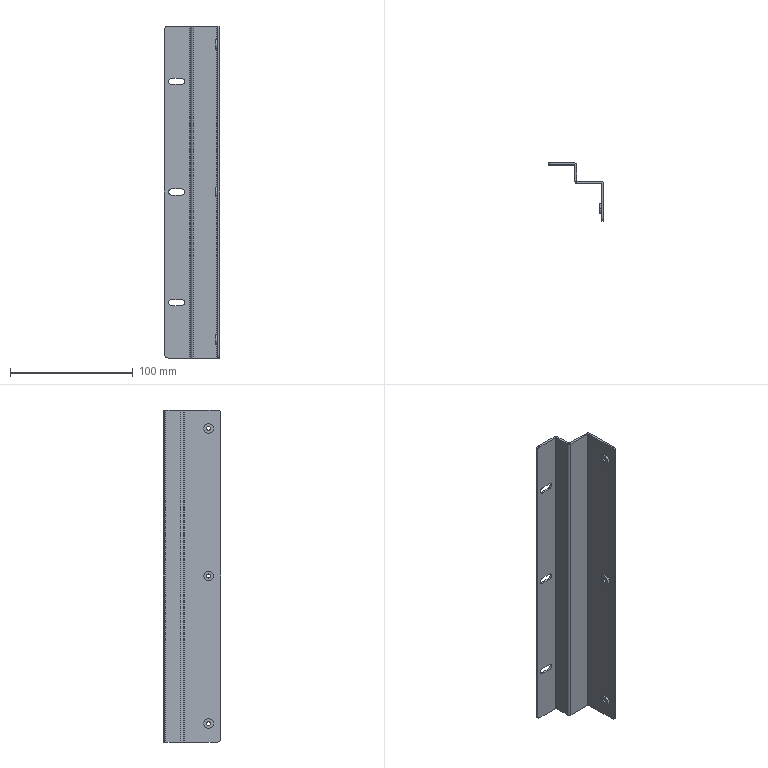Part | SolidWorks | features ICE 2, 3DProfileFeature 1, Fillet 1, FlatPattern 1, HoleWzd 1, SMBaseFlange 1, SheetMetal 1 | 1 solid | 61 faces | box 45 x 47 x 270 mm | volume 35809 mm3 | plane 33 | cylinder 28 | commonest cylinder face diameters 3.3 x6 5 x6 8 x6 6 x4 1.473 x3 4.473 x3